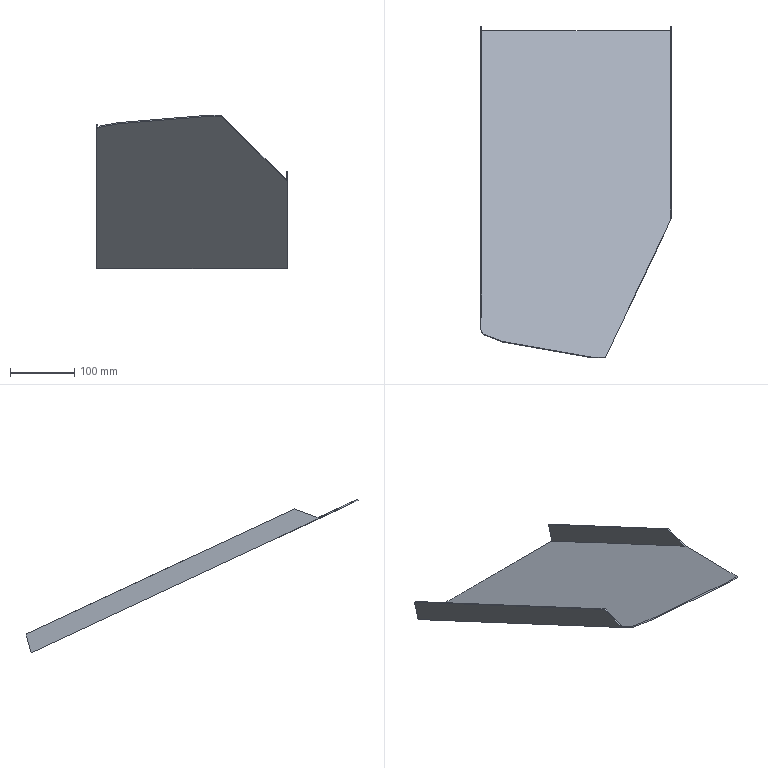Part | NX | features solid 2 | 1 solid | 16 faces | box 296.72 x 516.696 x 239.076 mm | volume 346164 mm3 | plane 16
STEP:
#1=CARTESIAN_POINT('',(393.683,810.204,-447.838));
#2=VERTEX_POINT('',#1);
#3=CARTESIAN_POINT('',(391.683,810.204,-447.838));
#4=VERTEX_POINT('',#3);
#5=CARTESIAN_POINT('',(393.683,810.204,-447.838));
#6=DIRECTION('',(-1.,0.,0.));
#7=VECTOR('',#6,1000.);
#8=LINE('',#5,#7);
#9=EDGE_CURVE('',#2,#4,#8,.T.);
#10=ORIENTED_EDGE('',*,*,#9,.F.);
#11=CARTESIAN_POINT('',(393.683,802.32,-477.263));
#12=VERTEX_POINT('',#11);
#13=CARTESIAN_POINT('',(393.683,816.816,-423.163));
#14=DIRECTION('',(0.,-0.2588,-0.9659));
#15=VECTOR('',#14,1000.);
#16=LINE('',#13,#15);
#17=EDGE_CURVE('',#2,#12,#16,.T.);
#18=ORIENTED_EDGE('',*,*,#17,.T.);
#19=CARTESIAN_POINT('',(96.964,802.32,-477.263));
#20=VERTEX_POINT('',#19);
#21=CARTESIAN_POINT('',(393.683,802.32,-477.263));
#22=DIRECTION('',(-1.,0.,0.));
#23=VECTOR('',#22,1000.);
#24=LINE('',#21,#23);
#25=EDGE_CURVE('',#20,#12,#24,.F.);
#26=ORIENTED_EDGE('',*,*,#25,.F.);
#27=CARTESIAN_POINT('',(96.964,810.204,-447.838));
#28=VERTEX_POINT('',#27);
#29=CARTESIAN_POINT('',(96.964,827.551,-383.097));
#30=DIRECTION('',(0.,-0.2588,-0.9659));
#31=VECTOR('',#30,1000.);
#32=LINE('',#29,#31);
#33=EDGE_CURVE('',#28,#20,#32,.T.);
#34=ORIENTED_EDGE('',*,*,#33,.F.);
#35=CARTESIAN_POINT('',(98.964,810.204,-447.838));
#36=VERTEX_POINT('',#35);
#37=CARTESIAN_POINT('',(86.964,810.204,-447.838));
#38=DIRECTION('',(-1.,0.,0.));
#39=VECTOR('',#38,1000.);
#40=LINE('',#37,#39);
#41=EDGE_CURVE('',#28,#36,#40,.F.);
#42=ORIENTED_EDGE('',*,*,#41,.T.);
#43=CARTESIAN_POINT('',(98.964,802.845,-475.301));
#44=VERTEX_POINT('',#43);
#45=CARTESIAN_POINT('',(98.964,824.507,-394.459));
#46=DIRECTION('',(0.,-0.2588,-0.9659));
#47=VECTOR('',#46,1000.);
#48=LINE('',#45,#47);
#49=EDGE_CURVE('',#36,#44,#48,.T.);
#50=ORIENTED_EDGE('',*,*,#49,.T.);
#51=CARTESIAN_POINT('',(391.683,802.845,-475.301));
#52=VERTEX_POINT('',#51);
#53=CARTESIAN_POINT('',(300.135,802.845,-475.301));
#54=DIRECTION('',(1.,0.,0.));
#55=VECTOR('',#54,1000.);
#56=LINE('',#53,#55);
#57=EDGE_CURVE('',#44,#52,#56,.T.);
#58=ORIENTED_EDGE('',*,*,#57,.T.);
#59=CARTESIAN_POINT('',(391.683,816.816,-423.163));
#60=DIRECTION('',(0.,-0.2588,-0.9659));
#61=VECTOR('',#60,1000.);
#62=LINE('',#59,#61);
#63=EDGE_CURVE('',#4,#52,#62,.T.);
#64=ORIENTED_EDGE('',*,*,#63,.F.);
#65=EDGE_LOOP('',(#10,#18,#26,#34,#42,#50,#58,#64));
#66=FACE_BOUND('',#65,.T.);
#67=CARTESIAN_POINT('',(86.964,801.152,-481.621));
#68=DIRECTION('',(0.,-0.9659,0.2588));
#69=DIRECTION('',(0.,-0.2588,-0.9659));
#70=AXIS2_PLACEMENT_3D('',#67,#68,#69);
#71=PLANE('',#70);
#72=ADVANCED_FACE('',(#66),#71,.F.);
#73=CARTESIAN_POINT('',(391.683,548.055,-325.596));
#74=VERTEX_POINT('',#73);
#75=CARTESIAN_POINT('',(391.683,522.679,-313.763));
#76=DIRECTION('',(0.,0.9063,-0.4226));
#77=VECTOR('',#76,1000.);
#78=LINE('',#75,#77);
#79=EDGE_CURVE('',#74,#4,#78,.T.);
#80=ORIENTED_EDGE('',*,*,#79,.T.);
#81=ORIENTED_EDGE('',*,*,#63,.T.);
#82=CARTESIAN_POINT('',(391.683,510.845,-339.139));
#83=VERTEX_POINT('',#82);
#84=CARTESIAN_POINT('',(391.683,510.845,-339.139));
#85=DIRECTION('',(0.,-0.9063,0.4226));
#86=VECTOR('',#85,1000.);
#87=LINE('',#84,#86);
#88=EDGE_CURVE('',#52,#83,#87,.T.);
#89=ORIENTED_EDGE('',*,*,#88,.T.);
#90=CARTESIAN_POINT('',(391.683,510.845,-339.139));
#91=DIRECTION('',(0.,-0.9397,-0.342));
#92=VECTOR('',#91,1000.);
#93=LINE('',#90,#92);
#94=EDGE_CURVE('',#83,#74,#93,.F.);
#95=ORIENTED_EDGE('',*,*,#94,.T.);
#96=EDGE_LOOP('',(#80,#81,#89,#95));
#97=FACE_BOUND('',#96,.T.);
#98=CARTESIAN_POINT('',(391.683,510.,-340.952));
#99=DIRECTION('',(1.,0.,0.));
#100=DIRECTION('',(0.,1.,0.));
#101=AXIS2_PLACEMENT_3D('',#98,#99,#100);
#102=PLANE('',#101);
#103=ADVANCED_FACE('',(#97),#102,.F.);
#104=CARTESIAN_POINT('',(96.964,337.076,-260.316));
#105=VERTEX_POINT('',#104);
#106=CARTESIAN_POINT('',(96.964,510.,-340.952));
#107=DIRECTION('',(0.,-0.9063,0.4226));
#108=VECTOR('',#107,1000.);
#109=LINE('',#106,#108);
#110=EDGE_CURVE('',#105,#20,#109,.F.);
#111=ORIENTED_EDGE('',*,*,#110,.T.);
#112=ORIENTED_EDGE('',*,*,#25,.T.);
#113=CARTESIAN_POINT('',(393.683,510.,-340.952));
#114=VERTEX_POINT('',#113);
#115=CARTESIAN_POINT('',(393.683,510.,-340.952));
#116=DIRECTION('',(0.,0.9063,-0.4226));
#117=VECTOR('',#116,1000.);
#118=LINE('',#115,#117);
#119=EDGE_CURVE('',#114,#12,#118,.T.);
#120=ORIENTED_EDGE('',*,*,#119,.F.);
#121=CARTESIAN_POINT('',(291.056,293.508,-240.));
#122=VERTEX_POINT('',#121);
#123=CARTESIAN_POINT('',(387.406,496.759,-334.777));
#124=DIRECTION('',(0.3947,0.8327,-0.3883));
#125=VECTOR('',#124,1000.);
#126=LINE('',#123,#125);
#127=EDGE_CURVE('',#122,#114,#126,.T.);
#128=ORIENTED_EDGE('',*,*,#127,.F.);
#129=CARTESIAN_POINT('',(271.342,293.508,-240.));
#130=VERTEX_POINT('',#129);
#131=CARTESIAN_POINT('',(300.135,293.508,-240.));
#132=DIRECTION('',(1.,0.,0.));
#133=VECTOR('',#132,1000.);
#134=LINE('',#131,#133);
#135=EDGE_CURVE('',#130,#122,#134,.T.);
#136=ORIENTED_EDGE('',*,*,#135,.F.);
#137=CARTESIAN_POINT('',(131.06,318.228,-251.527));
#138=VERTEX_POINT('',#137);
#139=CARTESIAN_POINT('',(131.06,318.228,-251.527));
#140=CARTESIAN_POINT('',(177.82,309.988,-247.685));
#141=CARTESIAN_POINT('',(224.581,301.748,-243.842));
#142=CARTESIAN_POINT('',(271.342,293.508,-240.));
#143=B_SPLINE_CURVE_WITH_KNOTS('',3,(#139,#140,#141,#142),.UNSPECIFIED.,.F.,.F.,(4,4),(0.,1.),.UNSPECIFIED.);
#144=EDGE_CURVE('',#138,#130,#143,.T.);
#145=ORIENTED_EDGE('',*,*,#144,.F.);
#146=CARTESIAN_POINT('',(101.092,329.717,-256.885));
#147=VERTEX_POINT('',#146);
#148=CARTESIAN_POINT('',(78.288,338.459,-260.961));
#149=DIRECTION('',(-0.921,0.3531,-0.1646));
#150=VECTOR('',#149,1000.);
#151=LINE('',#148,#150);
#152=EDGE_CURVE('',#138,#147,#151,.T.);
#153=ORIENTED_EDGE('',*,*,#152,.T.);
#154=CARTESIAN_POINT('',(119.676,296.588,-241.437));
#155=DIRECTION('',(0.4532,-0.8079,0.3767));
#156=VECTOR('',#155,1000.);
#157=LINE('',#154,#156);
#158=EDGE_CURVE('',#105,#147,#157,.T.);
#159=ORIENTED_EDGE('',*,*,#158,.F.);
#160=EDGE_LOOP('',(#111,#112,#120,#128,#136,#145,#153,#159));
#161=FACE_BOUND('',#160,.T.);
#162=CARTESIAN_POINT('',(393.683,510.,-340.952));
#163=DIRECTION('',(0.,-0.4226,-0.9063));
#164=DIRECTION('',(0.,0.9063,-0.4226));
#165=AXIS2_PLACEMENT_3D('',#162,#163,#164);
#166=PLANE('',#165);
#167=ADVANCED_FACE('',(#161),#166,.T.);
#168=CARTESIAN_POINT('',(393.683,548.055,-325.596));
#169=VERTEX_POINT('',#168);
#170=CARTESIAN_POINT('',(393.683,522.679,-313.763));
#171=DIRECTION('',(0.,0.9063,-0.4226));
#172=VECTOR('',#171,1000.);
#173=LINE('',#170,#172);
#174=EDGE_CURVE('',#169,#2,#173,.T.);
#175=ORIENTED_EDGE('',*,*,#174,.T.);
#176=ORIENTED_EDGE('',*,*,#9,.T.);
#177=ORIENTED_EDGE('',*,*,#79,.F.);
#178=CARTESIAN_POINT('',(393.683,548.055,-325.596));
#179=DIRECTION('',(1.,0.,0.));
#180=VECTOR('',#179,1000.);
#181=LINE('',#178,#180);
#182=EDGE_CURVE('',#74,#169,#181,.T.);
#183=ORIENTED_EDGE('',*,*,#182,.T.);
#184=EDGE_LOOP('',(#175,#176,#177,#183));
#185=FACE_BOUND('',#184,.T.);
#186=CARTESIAN_POINT('',(393.683,522.679,-313.763));
#187=DIRECTION('',(0.,-0.4226,-0.9063));
#188=DIRECTION('',(0.,0.9063,-0.4226));
#189=AXIS2_PLACEMENT_3D('',#186,#187,#188);
#190=PLANE('',#189);
#191=ADVANCED_FACE('',(#185),#190,.F.);
#192=ORIENTED_EDGE('',*,*,#17,.F.);
#193=ORIENTED_EDGE('',*,*,#174,.F.);
#194=CARTESIAN_POINT('',(393.683,510.845,-339.139));
#195=VERTEX_POINT('',#194);
#196=CARTESIAN_POINT('',(393.683,509.516,-339.623));
#197=DIRECTION('',(0.,0.9397,0.342));
#198=VECTOR('',#197,1000.);
#199=LINE('',#196,#198);
#200=EDGE_CURVE('',#169,#195,#199,.F.);
#201=ORIENTED_EDGE('',*,*,#200,.T.);
#202=CARTESIAN_POINT('',(393.683,510.,-340.952));
#203=DIRECTION('',(0.,0.4226,0.9063));
#204=VECTOR('',#203,1000.);
#205=LINE('',#202,#204);
#206=EDGE_CURVE('',#114,#195,#205,.T.);
#207=ORIENTED_EDGE('',*,*,#206,.F.);
#208=ORIENTED_EDGE('',*,*,#119,.T.);
#209=EDGE_LOOP('',(#192,#193,#201,#207,#208));
#210=FACE_BOUND('',#209,.T.);
#211=CARTESIAN_POINT('',(393.683,510.,-340.952));
#212=DIRECTION('',(1.,0.,0.));
#213=DIRECTION('',(0.,1.,0.));
#214=AXIS2_PLACEMENT_3D('',#211,#212,#213);
#215=PLANE('',#214);
#216=ADVANCED_FACE('',(#210),#215,.T.);
#217=ORIENTED_EDGE('',*,*,#200,.F.);
#218=ORIENTED_EDGE('',*,*,#182,.F.);
#219=ORIENTED_EDGE('',*,*,#94,.F.);
#220=CARTESIAN_POINT('',(393.683,510.845,-339.139));
#221=DIRECTION('',(-1.,0.,0.));
#222=VECTOR('',#221,1000.);
#223=LINE('',#220,#222);
#224=EDGE_CURVE('',#195,#83,#223,.T.);
#225=ORIENTED_EDGE('',*,*,#224,.F.);
#226=EDGE_LOOP('',(#217,#218,#219,#225));
#227=FACE_BOUND('',#226,.T.);
#228=CARTESIAN_POINT('',(393.683,510.845,-339.139));
#229=DIRECTION('',(0.,0.342,-0.9397));
#230=DIRECTION('',(0.,0.9397,0.342));
#231=AXIS2_PLACEMENT_3D('',#228,#229,#230);
#232=PLANE('',#231);
#233=ADVANCED_FACE('',(#227),#232,.F.);
#234=ORIENTED_EDGE('',*,*,#57,.F.);
#235=CARTESIAN_POINT('',(98.964,355.748,-266.816));
#236=VERTEX_POINT('',#235);
#237=CARTESIAN_POINT('',(98.964,294.353,-238.187));
#238=DIRECTION('',(0.,0.9063,-0.4226));
#239=VECTOR('',#238,1000.);
#240=LINE('',#237,#239);
#241=EDGE_CURVE('',#236,#44,#240,.T.);
#242=ORIENTED_EDGE('',*,*,#241,.F.);
#243=CARTESIAN_POINT('',(96.964,355.748,-266.816));
#244=VERTEX_POINT('',#243);
#245=CARTESIAN_POINT('',(86.964,355.748,-266.816));
#246=DIRECTION('',(1.,0.,0.));
#247=VECTOR('',#246,1000.);
#248=LINE('',#245,#247);
#249=EDGE_CURVE('',#236,#244,#248,.F.);
#250=ORIENTED_EDGE('',*,*,#249,.T.);
#251=CARTESIAN_POINT('',(96.964,337.922,-258.504));
#252=VERTEX_POINT('',#251);
#253=CARTESIAN_POINT('',(96.964,294.353,-238.187));
#254=DIRECTION('',(0.,-0.9063,0.4226));
#255=VECTOR('',#254,1000.);
#256=LINE('',#253,#255);
#257=EDGE_CURVE('',#244,#252,#256,.T.);
#258=ORIENTED_EDGE('',*,*,#257,.T.);
#259=CARTESIAN_POINT('',(101.092,330.562,-255.072));
#260=VERTEX_POINT('',#259);
#261=CARTESIAN_POINT('',(119.676,297.434,-239.624));
#262=DIRECTION('',(0.4532,-0.8079,0.3767));
#263=VECTOR('',#262,1000.);
#264=LINE('',#261,#263);
#265=EDGE_CURVE('',#252,#260,#264,.T.);
#266=ORIENTED_EDGE('',*,*,#265,.T.);
#267=CARTESIAN_POINT('',(131.06,319.073,-249.715));
#268=VERTEX_POINT('',#267);
#269=CARTESIAN_POINT('',(78.288,339.304,-259.148));
#270=DIRECTION('',(-0.921,0.3531,-0.1646));
#271=VECTOR('',#270,1000.);
#272=LINE('',#269,#271);
#273=EDGE_CURVE('',#268,#260,#272,.T.);
#274=ORIENTED_EDGE('',*,*,#273,.F.);
#275=CARTESIAN_POINT('',(271.342,294.353,-238.187));
#276=VERTEX_POINT('',#275);
#277=CARTESIAN_POINT('',(131.06,319.073,-249.715));
#278=CARTESIAN_POINT('',(177.82,310.833,-245.872));
#279=CARTESIAN_POINT('',(224.581,302.593,-242.03));
#280=CARTESIAN_POINT('',(271.342,294.353,-238.187));
#281=B_SPLINE_CURVE_WITH_KNOTS('',3,(#277,#278,#279,#280),.UNSPECIFIED.,.F.,.F.,(4,4),(0.,1.),.UNSPECIFIED.);
#282=EDGE_CURVE('',#268,#276,#281,.T.);
#283=ORIENTED_EDGE('',*,*,#282,.T.);
#284=CARTESIAN_POINT('',(291.056,294.353,-238.187));
#285=VERTEX_POINT('',#284);
#286=CARTESIAN_POINT('',(300.135,294.353,-238.187));
#287=DIRECTION('',(1.,0.,0.));
#288=VECTOR('',#287,1000.);
#289=LINE('',#286,#288);
#290=EDGE_CURVE('',#276,#285,#289,.T.);
#291=ORIENTED_EDGE('',*,*,#290,.T.);
#292=CARTESIAN_POINT('',(387.406,497.604,-332.965));
#293=DIRECTION('',(0.3947,0.8327,-0.3883));
#294=VECTOR('',#293,1000.);
#295=LINE('',#292,#294);
#296=EDGE_CURVE('',#285,#195,#295,.T.);
#297=ORIENTED_EDGE('',*,*,#296,.T.);
#298=ORIENTED_EDGE('',*,*,#224,.T.);
#299=ORIENTED_EDGE('',*,*,#88,.F.);
#300=EDGE_LOOP('',(#234,#242,#250,#258,#266,#274,#283,#291,#297,#298,#299));
#301=FACE_BOUND('',#300,.T.);
#302=CARTESIAN_POINT('',(300.135,294.353,-238.187));
#303=DIRECTION('',(0.,0.4226,0.9063));
#304=DIRECTION('',(1.,0.,0.));
#305=AXIS2_PLACEMENT_3D('',#302,#303,#304);
#306=PLANE('',#305);
#307=ADVANCED_FACE('',(#301),#306,.T.);
#308=CARTESIAN_POINT('',(96.964,392.958,-253.273));
#309=VERTEX_POINT('',#308);
#310=CARTESIAN_POINT('',(96.964,367.581,-241.44));
#311=DIRECTION('',(0.,-0.9063,0.4226));
#312=VECTOR('',#311,1000.);
#313=LINE('',#310,#312);
#314=EDGE_CURVE('',#309,#28,#313,.F.);
#315=ORIENTED_EDGE('',*,*,#314,.T.);
#316=ORIENTED_EDGE('',*,*,#33,.T.);
#317=ORIENTED_EDGE('',*,*,#110,.F.);
#318=CARTESIAN_POINT('',(96.964,337.076,-260.316));
#319=DIRECTION('',(0.,0.4226,0.9063));
#320=VECTOR('',#319,1000.);
#321=LINE('',#318,#320);
#322=EDGE_CURVE('',#105,#252,#321,.T.);
#323=ORIENTED_EDGE('',*,*,#322,.T.);
#324=ORIENTED_EDGE('',*,*,#257,.F.);
#325=CARTESIAN_POINT('',(96.964,392.958,-253.273));
#326=DIRECTION('',(0.,-0.9397,-0.342));
#327=VECTOR('',#326,1000.);
#328=LINE('',#325,#327);
#329=EDGE_CURVE('',#244,#309,#328,.F.);
#330=ORIENTED_EDGE('',*,*,#329,.T.);
#331=EDGE_LOOP('',(#315,#316,#317,#323,#324,#330));
#332=FACE_BOUND('',#331,.T.);
#333=CARTESIAN_POINT('',(96.964,293.508,-240.));
#334=DIRECTION('',(1.,0.,0.));
#335=DIRECTION('',(0.,1.,0.));
#336=AXIS2_PLACEMENT_3D('',#333,#334,#335);
#337=PLANE('',#336);
#338=ADVANCED_FACE('',(#332),#337,.F.);
#339=ORIENTED_EDGE('',*,*,#265,.F.);
#340=ORIENTED_EDGE('',*,*,#322,.F.);
#341=ORIENTED_EDGE('',*,*,#158,.T.);
#342=CARTESIAN_POINT('',(101.092,329.717,-256.885));
#343=DIRECTION('',(0.,0.4226,0.9063));
#344=VECTOR('',#343,1000.);
#345=LINE('',#342,#344);
#346=EDGE_CURVE('',#147,#260,#345,.T.);
#347=ORIENTED_EDGE('',*,*,#346,.T.);
#348=EDGE_LOOP('',(#339,#340,#341,#347));
#349=FACE_BOUND('',#348,.T.);
#350=CARTESIAN_POINT('',(119.676,296.588,-241.437));
#351=DIRECTION('',(-0.8914,-0.4107,0.1915));
#352=DIRECTION('',(0.4185,-0.9082,0.));
#353=AXIS2_PLACEMENT_3D('',#350,#351,#352);
#354=PLANE('',#353);
#355=ADVANCED_FACE('',(#349),#354,.T.);
#356=ORIENTED_EDGE('',*,*,#273,.T.);
#357=ORIENTED_EDGE('',*,*,#346,.F.);
#358=ORIENTED_EDGE('',*,*,#152,.F.);
#359=CARTESIAN_POINT('',(131.06,319.073,-249.715));
#360=CARTESIAN_POINT('',(131.06,318.792,-250.319));
#361=CARTESIAN_POINT('',(131.06,318.51,-250.923));
#362=CARTESIAN_POINT('',(131.06,318.228,-251.527));
#363=B_SPLINE_CURVE_WITH_KNOTS('',3,(#359,#360,#361,#362),.UNSPECIFIED.,.F.,.F.,(4,4),(0.,1.),.UNSPECIFIED.);
#364=EDGE_CURVE('',#138,#268,#363,.F.);
#365=ORIENTED_EDGE('',*,*,#364,.T.);
#366=EDGE_LOOP('',(#356,#357,#358,#365));
#367=FACE_BOUND('',#366,.T.);
#368=CARTESIAN_POINT('',(78.288,338.459,-260.961));
#369=DIRECTION('',(0.3896,0.8347,-0.3892));
#370=DIRECTION('',(-0.9062,0.4229,0.));
#371=AXIS2_PLACEMENT_3D('',#368,#369,#370);
#372=PLANE('',#371);
#373=ADVANCED_FACE('',(#367),#372,.F.);
#374=ORIENTED_EDGE('',*,*,#282,.F.);
#375=ORIENTED_EDGE('',*,*,#364,.F.);
#376=ORIENTED_EDGE('',*,*,#144,.T.);
#377=CARTESIAN_POINT('',(271.342,294.353,-238.187));
#378=CARTESIAN_POINT('',(271.342,294.071,-238.792));
#379=CARTESIAN_POINT('',(271.342,293.789,-239.396));
#380=CARTESIAN_POINT('',(271.342,293.508,-240.));
#381=B_SPLINE_CURVE_WITH_KNOTS('',3,(#377,#378,#379,#380),.UNSPECIFIED.,.F.,.F.,(4,4),(0.,1.),.UNSPECIFIED.);
#382=EDGE_CURVE('',#130,#276,#381,.F.);
#383=ORIENTED_EDGE('',*,*,#382,.T.);
#384=EDGE_LOOP('',(#374,#375,#376,#383));
#385=FACE_BOUND('',#384,.T.);
#386=CARTESIAN_POINT('',(131.06,318.228,-251.527));
#387=DIRECTION('',(-0.1909,-0.8896,0.4148));
#388=DIRECTION('',(0.,-0.4226,-0.9063));
#389=AXIS2_PLACEMENT_3D('',#386,#387,#388);
#390=PLANE('',#389);
#391=ADVANCED_FACE('',(#385),#390,.T.);
#392=ORIENTED_EDGE('',*,*,#290,.F.);
#393=ORIENTED_EDGE('',*,*,#382,.F.);
#394=ORIENTED_EDGE('',*,*,#135,.T.);
#395=CARTESIAN_POINT('',(291.056,293.508,-240.));
#396=DIRECTION('',(0.,0.4226,0.9063));
#397=VECTOR('',#396,1000.);
#398=LINE('',#395,#397);
#399=EDGE_CURVE('',#122,#285,#398,.T.);
#400=ORIENTED_EDGE('',*,*,#399,.T.);
#401=EDGE_LOOP('',(#392,#393,#394,#400));
#402=FACE_BOUND('',#401,.T.);
#403=CARTESIAN_POINT('',(300.135,293.508,-240.));
#404=DIRECTION('',(0.,-0.9063,0.4226));
#405=DIRECTION('',(0.,-0.4226,-0.9063));
#406=AXIS2_PLACEMENT_3D('',#403,#404,#405);
#407=PLANE('',#406);
#408=ADVANCED_FACE('',(#402),#407,.T.);
#409=ORIENTED_EDGE('',*,*,#296,.F.);
#410=ORIENTED_EDGE('',*,*,#399,.F.);
#411=ORIENTED_EDGE('',*,*,#127,.T.);
#412=ORIENTED_EDGE('',*,*,#206,.T.);
#413=EDGE_LOOP('',(#409,#410,#411,#412));
#414=FACE_BOUND('',#413,.T.);
#415=CARTESIAN_POINT('',(387.406,496.759,-334.777));
#416=DIRECTION('',(0.9188,-0.3578,0.1668));
#417=DIRECTION('',(0.3628,0.9319,0.));
#418=AXIS2_PLACEMENT_3D('',#415,#416,#417);
#419=PLANE('',#418);
#420=ADVANCED_FACE('',(#414),#419,.T.);
#421=ORIENTED_EDGE('',*,*,#49,.F.);
#422=CARTESIAN_POINT('',(98.964,392.958,-253.273));
#423=VERTEX_POINT('',#422);
#424=CARTESIAN_POINT('',(98.964,367.581,-241.44));
#425=DIRECTION('',(0.,-0.9063,0.4226));
#426=VECTOR('',#425,1000.);
#427=LINE('',#424,#426);
#428=EDGE_CURVE('',#423,#36,#427,.F.);
#429=ORIENTED_EDGE('',*,*,#428,.F.);
#430=CARTESIAN_POINT('',(98.964,354.419,-267.3));
#431=DIRECTION('',(0.,0.9397,0.342));
#432=VECTOR('',#431,1000.);
#433=LINE('',#430,#432);
#434=EDGE_CURVE('',#423,#236,#433,.F.);
#435=ORIENTED_EDGE('',*,*,#434,.T.);
#436=ORIENTED_EDGE('',*,*,#241,.T.);
#437=EDGE_LOOP('',(#421,#429,#435,#436));
#438=FACE_BOUND('',#437,.T.);
#439=CARTESIAN_POINT('',(98.964,354.903,-268.629));
#440=DIRECTION('',(1.,0.,0.));
#441=DIRECTION('',(0.,1.,0.));
#442=AXIS2_PLACEMENT_3D('',#439,#440,#441);
#443=PLANE('',#442);
#444=ADVANCED_FACE('',(#438),#443,.T.);
#445=ORIENTED_EDGE('',*,*,#41,.F.);
#446=ORIENTED_EDGE('',*,*,#314,.F.);
#447=CARTESIAN_POINT('',(86.964,392.958,-253.273));
#448=DIRECTION('',(-1.,0.,0.));
#449=VECTOR('',#448,1000.);
#450=LINE('',#447,#449);
#451=EDGE_CURVE('',#309,#423,#450,.F.);
#452=ORIENTED_EDGE('',*,*,#451,.T.);
#453=ORIENTED_EDGE('',*,*,#428,.T.);
#454=EDGE_LOOP('',(#445,#446,#452,#453));
#455=FACE_BOUND('',#454,.T.);
#456=CARTESIAN_POINT('',(86.964,367.581,-241.44));
#457=DIRECTION('',(0.,-0.4226,-0.9063));
#458=DIRECTION('',(0.,0.9063,-0.4226));
#459=AXIS2_PLACEMENT_3D('',#456,#457,#458);
#460=PLANE('',#459);
#461=ADVANCED_FACE('',(#455),#460,.F.);
#462=ORIENTED_EDGE('',*,*,#329,.F.);
#463=ORIENTED_EDGE('',*,*,#249,.F.);
#464=ORIENTED_EDGE('',*,*,#434,.F.);
#465=ORIENTED_EDGE('',*,*,#451,.F.);
#466=EDGE_LOOP('',(#462,#463,#464,#465));
#467=FACE_BOUND('',#466,.T.);
#468=CARTESIAN_POINT('',(86.964,392.958,-253.273));
#469=DIRECTION('',(0.,0.342,-0.9397));
#470=DIRECTION('',(0.,0.9397,0.342));
#471=AXIS2_PLACEMENT_3D('',#468,#469,#470);
#472=PLANE('',#471);
#473=ADVANCED_FACE('',(#467),#472,.F.);
#474=CLOSED_SHELL('',(#72,#103,#167,#191,#216,#233,#307,#338,#355,#373,#391,#408,#420,#444,#461,#473));
#475=MANIFOLD_SOLID_BREP('',#474);
#476=(LENGTH_UNIT()NAMED_UNIT(*)SI_UNIT(.MILLI.,.METRE.));
#477=UNCERTAINTY_MEASURE_WITH_UNIT(LENGTH_MEASURE(0.0508),#476,'','');
#478=(NAMED_UNIT(*)PLANE_ANGLE_UNIT()SI_UNIT($,.RADIAN.));
#479=(NAMED_UNIT(*)SI_UNIT($,.STERADIAN.)SOLID_ANGLE_UNIT());
#480=(GEOMETRIC_REPRESENTATION_CONTEXT(3)GLOBAL_UNCERTAINTY_ASSIGNED_CONTEXT((#477))GLOBAL_UNIT_ASSIGNED_CONTEXT((#476,#478,#479))REPRESENTATION_CONTEXT('',''));
#481=ADVANCED_BREP_SHAPE_REPRESENTATION('',(#475),#480);